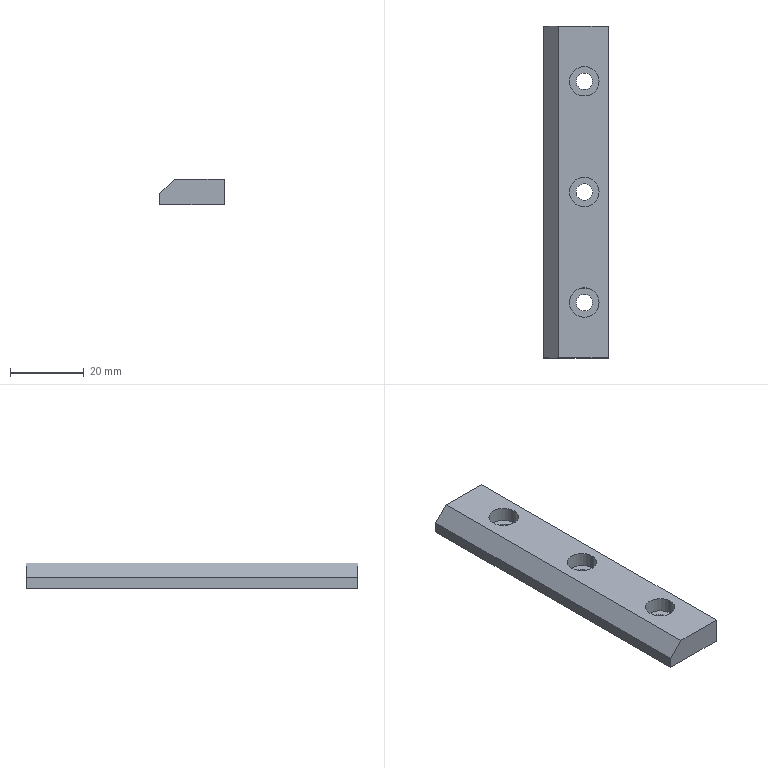Part | STEP file | detection slide seat cover plate--1 | 1 solid | 22 faces | box 17.5 x 90 x 7 mm | volume 9559 mm3 | cylinder 12 | plane 10 | commonest cylinder face diameters 4.5 x6 8 x6
STEP:
#1=CARTESIAN_POINT('',(0.,0.,0.));
#2=DIRECTION('',(0.,0.,1.));
#3=DIRECTION('',(1.,0.,0.));
#4=AXIS2_PLACEMENT_3D('',#1,#2,#3);
#5=CARTESIAN_POINT('',(7.648,22.1,3.));
#6=VERTEX_POINT('',#5);
#7=CARTESIAN_POINT('',(7.648,22.1,7.));
#8=VERTEX_POINT('',#7);
#9=CARTESIAN_POINT('',(7.648,22.1,3.));
#10=DIRECTION('',(0.,0.,1.));
#11=VECTOR('',#10,1.);
#12=LINE('',#9,#11);
#13=CARTESIAN_POINT('',(3.648,22.1,3.));
#14=DIRECTION('',(0.,0.,1.));
#15=DIRECTION('',(1.,0.,0.));
#16=AXIS2_PLACEMENT_3D('',#13,#14,#15);
#17=CYLINDRICAL_SURFACE('',#16,4.);
#18=CARTESIAN_POINT('',(6.283,0.));
#19=DIRECTION('',(0.,1.));
#20=VECTOR('',#19,1.);
#21=LINE('',#18,#20);
#22=(GEOMETRIC_REPRESENTATION_CONTEXT(2)PARAMETRIC_REPRESENTATION_CONTEXT()REPRESENTATION_CONTEXT('',''));
#23=DEFINITIONAL_REPRESENTATION('',(#21),#22);
#24=PCURVE('',#17,#23);
#25=CARTESIAN_POINT('',(3.648,22.1,3.));
#26=DIRECTION('',(0.,0.,1.));
#27=DIRECTION('',(1.,0.,0.));
#28=AXIS2_PLACEMENT_3D('',#25,#26,#27);
#29=CYLINDRICAL_SURFACE('',#28,4.);
#30=CARTESIAN_POINT('',(0.,0.));
#31=DIRECTION('',(0.,1.));
#32=VECTOR('',#31,1.);
#33=LINE('',#30,#32);
#34=(GEOMETRIC_REPRESENTATION_CONTEXT(2)PARAMETRIC_REPRESENTATION_CONTEXT()REPRESENTATION_CONTEXT('',''));
#35=DEFINITIONAL_REPRESENTATION('',(#33),#34);
#36=PCURVE('',#29,#35);
#37=SURFACE_CURVE('',#12,(#24,#36),.PCURVE_S1.);
#38=EDGE_CURVE('',#6,#8,#37,.T.);
#39=ORIENTED_EDGE('',*,*,#38,.T.);
#40=CARTESIAN_POINT('',(-0.3518,22.1,7.));
#41=VERTEX_POINT('',#40);
#42=CARTESIAN_POINT('',(3.648,22.1,7.));
#43=DIRECTION('',(0.,0.,1.));
#44=DIRECTION('',(1.,0.,0.));
#45=AXIS2_PLACEMENT_3D('',#42,#43,#44);
#46=CIRCLE('',#45,4.);
#47=CARTESIAN_POINT('',(0.,4.));
#48=DIRECTION('',(1.,0.));
#49=VECTOR('',#48,1.);
#50=LINE('',#47,#49);
#51=(GEOMETRIC_REPRESENTATION_CONTEXT(2)PARAMETRIC_REPRESENTATION_CONTEXT()REPRESENTATION_CONTEXT('',''));
#52=DEFINITIONAL_REPRESENTATION('',(#50),#51);
#53=PCURVE('',#17,#52);
#54=CARTESIAN_POINT('',(-7.352,-52.9,7.));
#55=DIRECTION('',(0.,0.,1.));
#56=DIRECTION('',(1.,0.,0.));
#57=AXIS2_PLACEMENT_3D('',#54,#55,#56);
#58=PLANE('',#57);
#59=CARTESIAN_POINT('',(11.,75.));
#60=DIRECTION('',(1.,0.));
#61=AXIS2_PLACEMENT_2D('',#59,#60);
#62=CIRCLE('',#61,4.);
#63=(GEOMETRIC_REPRESENTATION_CONTEXT(2)PARAMETRIC_REPRESENTATION_CONTEXT()REPRESENTATION_CONTEXT('',''));
#64=DEFINITIONAL_REPRESENTATION('',(#62),#63);
#65=PCURVE('',#58,#64);
#66=SURFACE_CURVE('',#46,(#53,#65),.PCURVE_S1.);
#67=EDGE_CURVE('',#41,#8,#66,.T.);
#68=ORIENTED_EDGE('',*,*,#67,.F.);
#69=CARTESIAN_POINT('',(-0.3518,22.1,3.));
#70=VERTEX_POINT('',#69);
#71=CARTESIAN_POINT('',(-0.3518,22.1,3.));
#72=DIRECTION('',(0.,0.,1.));
#73=VECTOR('',#72,1.);
#74=LINE('',#71,#73);
#75=CARTESIAN_POINT('',(3.142,0.));
#76=DIRECTION('',(0.,1.));
#77=VECTOR('',#76,1.);
#78=LINE('',#75,#77);
#79=(GEOMETRIC_REPRESENTATION_CONTEXT(2)PARAMETRIC_REPRESENTATION_CONTEXT()REPRESENTATION_CONTEXT('',''));
#80=DEFINITIONAL_REPRESENTATION('',(#78),#79);
#81=PCURVE('',#17,#80);
#82=CARTESIAN_POINT('',(3.142,0.));
#83=DIRECTION('',(0.,1.));
#84=VECTOR('',#83,1.);
#85=LINE('',#82,#84);
#86=(GEOMETRIC_REPRESENTATION_CONTEXT(2)PARAMETRIC_REPRESENTATION_CONTEXT()REPRESENTATION_CONTEXT('',''));
#87=DEFINITIONAL_REPRESENTATION('',(#85),#86);
#88=PCURVE('',#29,#87);
#89=SURFACE_CURVE('',#74,(#81,#88),.PCURVE_S1.);
#90=EDGE_CURVE('',#70,#41,#89,.T.);
#91=ORIENTED_EDGE('',*,*,#90,.F.);
#92=CARTESIAN_POINT('',(3.648,22.1,3.));
#93=DIRECTION('',(0.,0.,1.));
#94=DIRECTION('',(1.,0.,0.));
#95=AXIS2_PLACEMENT_3D('',#92,#93,#94);
#96=CIRCLE('',#95,4.);
#97=CARTESIAN_POINT('',(0.,0.));
#98=DIRECTION('',(1.,0.));
#99=VECTOR('',#98,1.);
#100=LINE('',#97,#99);
#101=(GEOMETRIC_REPRESENTATION_CONTEXT(2)PARAMETRIC_REPRESENTATION_CONTEXT()REPRESENTATION_CONTEXT('',''));
#102=DEFINITIONAL_REPRESENTATION('',(#100),#101);
#103=PCURVE('',#17,#102);
#104=CARTESIAN_POINT('',(3.648,22.1,3.));
#105=DIRECTION('',(0.,0.,1.));
#106=DIRECTION('',(1.,0.,0.));
#107=AXIS2_PLACEMENT_3D('',#104,#105,#106);
#108=PLANE('',#107);
#109=CARTESIAN_POINT('',(0.,0.));
#110=DIRECTION('',(1.,0.));
#111=AXIS2_PLACEMENT_2D('',#109,#110);
#112=CIRCLE('',#111,4.);
#113=(GEOMETRIC_REPRESENTATION_CONTEXT(2)PARAMETRIC_REPRESENTATION_CONTEXT()REPRESENTATION_CONTEXT('',''));
#114=DEFINITIONAL_REPRESENTATION('',(#112),#113);
#115=PCURVE('',#108,#114);
#116=SURFACE_CURVE('',#96,(#103,#115),.PCURVE_S1.);
#117=EDGE_CURVE('',#70,#6,#116,.T.);
#118=ORIENTED_EDGE('',*,*,#117,.T.);
#119=EDGE_LOOP('',(#39,#68,#91,#118));
#120=FACE_BOUND('',#119,.F.);
#121=ADVANCED_FACE('',(#120),#17,.F.);
#122=CARTESIAN_POINT('',(7.648,-7.9,3.));
#123=VERTEX_POINT('',#122);
#124=CARTESIAN_POINT('',(7.648,-7.9,7.));
#125=VERTEX_POINT('',#124);
#126=CARTESIAN_POINT('',(7.648,-7.9,3.));
#127=DIRECTION('',(0.,0.,1.));
#128=VECTOR('',#127,1.);
#129=LINE('',#126,#128);
#130=CARTESIAN_POINT('',(3.648,-7.9,3.));
#131=DIRECTION('',(0.,0.,1.));
#132=DIRECTION('',(1.,0.,0.));
#133=AXIS2_PLACEMENT_3D('',#130,#131,#132);
#134=CYLINDRICAL_SURFACE('',#133,4.);
#135=CARTESIAN_POINT('',(6.283,0.));
#136=DIRECTION('',(0.,1.));
#137=VECTOR('',#136,1.);
#138=LINE('',#135,#137);
#139=(GEOMETRIC_REPRESENTATION_CONTEXT(2)PARAMETRIC_REPRESENTATION_CONTEXT()REPRESENTATION_CONTEXT('',''));
#140=DEFINITIONAL_REPRESENTATION('',(#138),#139);
#141=PCURVE('',#134,#140);
#142=CARTESIAN_POINT('',(3.648,-7.9,3.));
#143=DIRECTION('',(0.,0.,1.));
#144=DIRECTION('',(1.,0.,0.));
#145=AXIS2_PLACEMENT_3D('',#142,#143,#144);
#146=CYLINDRICAL_SURFACE('',#145,4.);
#147=CARTESIAN_POINT('',(0.,0.));
#148=DIRECTION('',(0.,1.));
#149=VECTOR('',#148,1.);
#150=LINE('',#147,#149);
#151=(GEOMETRIC_REPRESENTATION_CONTEXT(2)PARAMETRIC_REPRESENTATION_CONTEXT()REPRESENTATION_CONTEXT('',''));
#152=DEFINITIONAL_REPRESENTATION('',(#150),#151);
#153=PCURVE('',#146,#152);
#154=SURFACE_CURVE('',#129,(#141,#153),.PCURVE_S1.);
#155=EDGE_CURVE('',#123,#125,#154,.T.);
#156=ORIENTED_EDGE('',*,*,#155,.T.);
#157=CARTESIAN_POINT('',(-0.3518,-7.9,7.));
#158=VERTEX_POINT('',#157);
#159=CARTESIAN_POINT('',(3.648,-7.9,7.));
#160=DIRECTION('',(0.,0.,1.));
#161=DIRECTION('',(1.,0.,0.));
#162=AXIS2_PLACEMENT_3D('',#159,#160,#161);
#163=CIRCLE('',#162,4.);
#164=CARTESIAN_POINT('',(0.,4.));
#165=DIRECTION('',(1.,0.));
#166=VECTOR('',#165,1.);
#167=LINE('',#164,#166);
#168=(GEOMETRIC_REPRESENTATION_CONTEXT(2)PARAMETRIC_REPRESENTATION_CONTEXT()REPRESENTATION_CONTEXT('',''));
#169=DEFINITIONAL_REPRESENTATION('',(#167),#168);
#170=PCURVE('',#134,#169);
#171=CARTESIAN_POINT('',(11.,45.));
#172=DIRECTION('',(1.,0.));
#173=AXIS2_PLACEMENT_2D('',#171,#172);
#174=CIRCLE('',#173,4.);
#175=(GEOMETRIC_REPRESENTATION_CONTEXT(2)PARAMETRIC_REPRESENTATION_CONTEXT()REPRESENTATION_CONTEXT('',''));
#176=DEFINITIONAL_REPRESENTATION('',(#174),#175);
#177=PCURVE('',#58,#176);
#178=SURFACE_CURVE('',#163,(#170,#177),.PCURVE_S1.);
#179=EDGE_CURVE('',#158,#125,#178,.T.);
#180=ORIENTED_EDGE('',*,*,#179,.F.);
#181=CARTESIAN_POINT('',(-0.3518,-7.9,3.));
#182=VERTEX_POINT('',#181);
#183=CARTESIAN_POINT('',(-0.3518,-7.9,3.));
#184=DIRECTION('',(0.,0.,1.));
#185=VECTOR('',#184,1.);
#186=LINE('',#183,#185);
#187=CARTESIAN_POINT('',(3.142,0.));
#188=DIRECTION('',(0.,1.));
#189=VECTOR('',#188,1.);
#190=LINE('',#187,#189);
#191=(GEOMETRIC_REPRESENTATION_CONTEXT(2)PARAMETRIC_REPRESENTATION_CONTEXT()REPRESENTATION_CONTEXT('',''));
#192=DEFINITIONAL_REPRESENTATION('',(#190),#191);
#193=PCURVE('',#134,#192);
#194=CARTESIAN_POINT('',(3.142,0.));
#195=DIRECTION('',(0.,1.));
#196=VECTOR('',#195,1.);
#197=LINE('',#194,#196);
#198=(GEOMETRIC_REPRESENTATION_CONTEXT(2)PARAMETRIC_REPRESENTATION_CONTEXT()REPRESENTATION_CONTEXT('',''));
#199=DEFINITIONAL_REPRESENTATION('',(#197),#198);
#200=PCURVE('',#146,#199);
#201=SURFACE_CURVE('',#186,(#193,#200),.PCURVE_S1.);
#202=EDGE_CURVE('',#182,#158,#201,.T.);
#203=ORIENTED_EDGE('',*,*,#202,.F.);
#204=CARTESIAN_POINT('',(3.648,-7.9,3.));
#205=DIRECTION('',(0.,0.,1.));
#206=DIRECTION('',(1.,0.,0.));
#207=AXIS2_PLACEMENT_3D('',#204,#205,#206);
#208=CIRCLE('',#207,4.);
#209=CARTESIAN_POINT('',(0.,0.));
#210=DIRECTION('',(1.,0.));
#211=VECTOR('',#210,1.);
#212=LINE('',#209,#211);
#213=(GEOMETRIC_REPRESENTATION_CONTEXT(2)PARAMETRIC_REPRESENTATION_CONTEXT()REPRESENTATION_CONTEXT('',''));
#214=DEFINITIONAL_REPRESENTATION('',(#212),#213);
#215=PCURVE('',#134,#214);
#216=CARTESIAN_POINT('',(3.648,-7.9,3.));
#217=DIRECTION('',(0.,0.,1.));
#218=DIRECTION('',(1.,0.,0.));
#219=AXIS2_PLACEMENT_3D('',#216,#217,#218);
#220=PLANE('',#219);
#221=CARTESIAN_POINT('',(0.,0.));
#222=DIRECTION('',(1.,0.));
#223=AXIS2_PLACEMENT_2D('',#221,#222);
#224=CIRCLE('',#223,4.);
#225=(GEOMETRIC_REPRESENTATION_CONTEXT(2)PARAMETRIC_REPRESENTATION_CONTEXT()REPRESENTATION_CONTEXT('',''));
#226=DEFINITIONAL_REPRESENTATION('',(#224),#225);
#227=PCURVE('',#220,#226);
#228=SURFACE_CURVE('',#208,(#215,#227),.PCURVE_S1.);
#229=EDGE_CURVE('',#182,#123,#228,.T.);
#230=ORIENTED_EDGE('',*,*,#229,.T.);
#231=EDGE_LOOP('',(#156,#180,#203,#230));
#232=FACE_BOUND('',#231,.F.);
#233=ADVANCED_FACE('',(#232),#134,.F.);
#234=CARTESIAN_POINT('',(7.648,-37.9,3.));
#235=VERTEX_POINT('',#234);
#236=CARTESIAN_POINT('',(7.648,-37.9,7.));
#237=VERTEX_POINT('',#236);
#238=CARTESIAN_POINT('',(7.648,-37.9,3.));
#239=DIRECTION('',(0.,0.,1.));
#240=VECTOR('',#239,1.);
#241=LINE('',#238,#240);
#242=CARTESIAN_POINT('',(3.648,-37.9,3.));
#243=DIRECTION('',(0.,0.,1.));
#244=DIRECTION('',(1.,0.,0.));
#245=AXIS2_PLACEMENT_3D('',#242,#243,#244);
#246=CYLINDRICAL_SURFACE('',#245,4.);
#247=CARTESIAN_POINT('',(6.283,0.));
#248=DIRECTION('',(0.,1.));
#249=VECTOR('',#248,1.);
#250=LINE('',#247,#249);
#251=(GEOMETRIC_REPRESENTATION_CONTEXT(2)PARAMETRIC_REPRESENTATION_CONTEXT()REPRESENTATION_CONTEXT('',''));
#252=DEFINITIONAL_REPRESENTATION('',(#250),#251);
#253=PCURVE('',#246,#252);
#254=CARTESIAN_POINT('',(3.648,-37.9,3.));
#255=DIRECTION('',(0.,0.,1.));
#256=DIRECTION('',(1.,0.,0.));
#257=AXIS2_PLACEMENT_3D('',#254,#255,#256);
#258=CYLINDRICAL_SURFACE('',#257,4.);
#259=CARTESIAN_POINT('',(0.,0.));
#260=DIRECTION('',(0.,1.));
#261=VECTOR('',#260,1.);
#262=LINE('',#259,#261);
#263=(GEOMETRIC_REPRESENTATION_CONTEXT(2)PARAMETRIC_REPRESENTATION_CONTEXT()REPRESENTATION_CONTEXT('',''));
#264=DEFINITIONAL_REPRESENTATION('',(#262),#263);
#265=PCURVE('',#258,#264);
#266=SURFACE_CURVE('',#241,(#253,#265),.PCURVE_S1.);
#267=EDGE_CURVE('',#235,#237,#266,.T.);
#268=ORIENTED_EDGE('',*,*,#267,.T.);
#269=CARTESIAN_POINT('',(-0.3518,-37.9,7.));
#270=VERTEX_POINT('',#269);
#271=CARTESIAN_POINT('',(3.648,-37.9,7.));
#272=DIRECTION('',(0.,0.,1.));
#273=DIRECTION('',(1.,0.,0.));
#274=AXIS2_PLACEMENT_3D('',#271,#272,#273);
#275=CIRCLE('',#274,4.);
#276=CARTESIAN_POINT('',(0.,4.));
#277=DIRECTION('',(1.,0.));
#278=VECTOR('',#277,1.);
#279=LINE('',#276,#278);
#280=(GEOMETRIC_REPRESENTATION_CONTEXT(2)PARAMETRIC_REPRESENTATION_CONTEXT()REPRESENTATION_CONTEXT('',''));
#281=DEFINITIONAL_REPRESENTATION('',(#279),#280);
#282=PCURVE('',#246,#281);
#283=CARTESIAN_POINT('',(11.,15.));
#284=DIRECTION('',(1.,0.));
#285=AXIS2_PLACEMENT_2D('',#283,#284);
#286=CIRCLE('',#285,4.);
#287=(GEOMETRIC_REPRESENTATION_CONTEXT(2)PARAMETRIC_REPRESENTATION_CONTEXT()REPRESENTATION_CONTEXT('',''));
#288=DEFINITIONAL_REPRESENTATION('',(#286),#287);
#289=PCURVE('',#58,#288);
#290=SURFACE_CURVE('',#275,(#282,#289),.PCURVE_S1.);
#291=EDGE_CURVE('',#270,#237,#290,.T.);
#292=ORIENTED_EDGE('',*,*,#291,.F.);
#293=CARTESIAN_POINT('',(-0.3518,-37.9,3.));
#294=VERTEX_POINT('',#293);
#295=CARTESIAN_POINT('',(-0.3518,-37.9,3.));
#296=DIRECTION('',(0.,0.,1.));
#297=VECTOR('',#296,1.);
#298=LINE('',#295,#297);
#299=CARTESIAN_POINT('',(3.142,0.));
#300=DIRECTION('',(0.,1.));
#301=VECTOR('',#300,1.);
#302=LINE('',#299,#301);
#303=(GEOMETRIC_REPRESENTATION_CONTEXT(2)PARAMETRIC_REPRESENTATION_CONTEXT()REPRESENTATION_CONTEXT('',''));
#304=DEFINITIONAL_REPRESENTATION('',(#302),#303);
#305=PCURVE('',#246,#304);
#306=CARTESIAN_POINT('',(3.142,0.));
#307=DIRECTION('',(0.,1.));
#308=VECTOR('',#307,1.);
#309=LINE('',#306,#308);
#310=(GEOMETRIC_REPRESENTATION_CONTEXT(2)PARAMETRIC_REPRESENTATION_CONTEXT()REPRESENTATION_CONTEXT('',''));
#311=DEFINITIONAL_REPRESENTATION('',(#309),#310);
#312=PCURVE('',#258,#311);
#313=SURFACE_CURVE('',#298,(#305,#312),.PCURVE_S1.);
#314=EDGE_CURVE('',#294,#270,#313,.T.);
#315=ORIENTED_EDGE('',*,*,#314,.F.);
#316=CARTESIAN_POINT('',(3.648,-37.9,3.));
#317=DIRECTION('',(0.,0.,1.));
#318=DIRECTION('',(1.,0.,0.));
#319=AXIS2_PLACEMENT_3D('',#316,#317,#318);
#320=CIRCLE('',#319,4.);
#321=CARTESIAN_POINT('',(0.,0.));
#322=DIRECTION('',(1.,0.));
#323=VECTOR('',#322,1.);
#324=LINE('',#321,#323);
#325=(GEOMETRIC_REPRESENTATION_CONTEXT(2)PARAMETRIC_REPRESENTATION_CONTEXT()REPRESENTATION_CONTEXT('',''));
#326=DEFINITIONAL_REPRESENTATION('',(#324),#325);
#327=PCURVE('',#246,#326);
#328=CARTESIAN_POINT('',(3.648,-37.9,3.));
#329=DIRECTION('',(0.,0.,1.));
#330=DIRECTION('',(1.,0.,0.));
#331=AXIS2_PLACEMENT_3D('',#328,#329,#330);
#332=PLANE('',#331);
#333=CARTESIAN_POINT('',(0.,0.));
#334=DIRECTION('',(1.,0.));
#335=AXIS2_PLACEMENT_2D('',#333,#334);
#336=CIRCLE('',#335,4.);
#337=(GEOMETRIC_REPRESENTATION_CONTEXT(2)PARAMETRIC_REPRESENTATION_CONTEXT()REPRESENTATION_CONTEXT('',''));
#338=DEFINITIONAL_REPRESENTATION('',(#336),#337);
#339=PCURVE('',#332,#338);
#340=SURFACE_CURVE('',#320,(#327,#339),.PCURVE_S1.);
#341=EDGE_CURVE('',#294,#235,#340,.T.);
#342=ORIENTED_EDGE('',*,*,#341,.T.);
#343=EDGE_LOOP('',(#268,#292,#315,#342));
#344=FACE_BOUND('',#343,.F.);
#345=ADVANCED_FACE('',(#344),#246,.F.);
#346=CARTESIAN_POINT('',(1.398,-37.9,3.));
#347=VERTEX_POINT('',#346);
#348=CARTESIAN_POINT('',(1.398,-37.9,0.));
#349=VERTEX_POINT('',#348);
#350=CARTESIAN_POINT('',(1.398,-37.9,7.));
#351=DIRECTION('',(0.,0.,-1.));
#352=VECTOR('',#351,1.);
#353=LINE('',#350,#352);
#354=CARTESIAN_POINT('',(3.648,-37.9,7.));
#355=DIRECTION('',(0.,0.,-1.));
#356=DIRECTION('',(-1.,0.,0.));
#357=AXIS2_PLACEMENT_3D('',#354,#355,#356);
#358=CYLINDRICAL_SURFACE('',#357,2.25);
#359=CARTESIAN_POINT('',(6.283,0.));
#360=DIRECTION('',(0.,1.));
#361=VECTOR('',#360,1.);
#362=LINE('',#359,#361);
#363=(GEOMETRIC_REPRESENTATION_CONTEXT(2)PARAMETRIC_REPRESENTATION_CONTEXT()REPRESENTATION_CONTEXT('',''));
#364=DEFINITIONAL_REPRESENTATION('',(#362),#363);
#365=PCURVE('',#358,#364);
#366=CARTESIAN_POINT('',(3.648,-37.9,7.));
#367=DIRECTION('',(0.,0.,-1.));
#368=DIRECTION('',(-1.,0.,0.));
#369=AXIS2_PLACEMENT_3D('',#366,#367,#368);
#370=CYLINDRICAL_SURFACE('',#369,2.25);
#371=CARTESIAN_POINT('',(0.,0.));
#372=DIRECTION('',(0.,1.));
#373=VECTOR('',#372,1.);
#374=LINE('',#371,#373);
#375=(GEOMETRIC_REPRESENTATION_CONTEXT(2)PARAMETRIC_REPRESENTATION_CONTEXT()REPRESENTATION_CONTEXT('',''));
#376=DEFINITIONAL_REPRESENTATION('',(#374),#375);
#377=PCURVE('',#370,#376);
#378=SURFACE_CURVE('',#353,(#365,#377),.PCURVE_S1.);
#379=EDGE_CURVE('',#347,#349,#378,.T.);
#380=ORIENTED_EDGE('',*,*,#379,.T.);
#381=CARTESIAN_POINT('',(5.898,-37.9,0.));
#382=VERTEX_POINT('',#381);
#383=CARTESIAN_POINT('',(3.648,-37.9,0.));
#384=DIRECTION('',(0.,0.,1.));
#385=DIRECTION('',(1.,0.,0.));
#386=AXIS2_PLACEMENT_3D('',#383,#384,#385);
#387=CIRCLE('',#386,2.25);
#388=CARTESIAN_POINT('',(9.425,7.));
#389=DIRECTION('',(-1.,0.));
#390=VECTOR('',#389,1.);
#391=LINE('',#388,#390);
#392=(GEOMETRIC_REPRESENTATION_CONTEXT(2)PARAMETRIC_REPRESENTATION_CONTEXT()REPRESENTATION_CONTEXT('',''));
#393=DEFINITIONAL_REPRESENTATION('',(#391),#392);
#394=PCURVE('',#358,#393);
#395=CARTESIAN_POINT('',(-7.352,-52.9,0.));
#396=DIRECTION('',(0.,0.,1.));
#397=DIRECTION('',(1.,0.,0.));
#398=AXIS2_PLACEMENT_3D('',#395,#396,#397);
#399=PLANE('',#398);
#400=CARTESIAN_POINT('',(11.,15.));
#401=DIRECTION('',(1.,0.));
#402=AXIS2_PLACEMENT_2D('',#400,#401);
#403=CIRCLE('',#402,2.25);
#404=(GEOMETRIC_REPRESENTATION_CONTEXT(2)PARAMETRIC_REPRESENTATION_CONTEXT()REPRESENTATION_CONTEXT('',''));
#405=DEFINITIONAL_REPRESENTATION('',(#403),#404);
#406=PCURVE('',#399,#405);
#407=SURFACE_CURVE('',#387,(#394,#406),.PCURVE_S1.);
#408=EDGE_CURVE('',#349,#382,#407,.T.);
#409=ORIENTED_EDGE('',*,*,#408,.T.);
#410=CARTESIAN_POINT('',(5.898,-37.9,3.));
#411=VERTEX_POINT('',#410);
#412=CARTESIAN_POINT('',(5.898,-37.9,7.));
#413=DIRECTION('',(0.,0.,-1.));
#414=VECTOR('',#413,1.);
#415=LINE('',#412,#414);
#416=CARTESIAN_POINT('',(3.142,0.));
#417=DIRECTION('',(0.,1.));
#418=VECTOR('',#417,1.);
#419=LINE('',#416,#418);
#420=(GEOMETRIC_REPRESENTATION_CONTEXT(2)PARAMETRIC_REPRESENTATION_CONTEXT()REPRESENTATION_CONTEXT('',''));
#421=DEFINITIONAL_REPRESENTATION('',(#419),#420);
#422=PCURVE('',#358,#421);
#423=CARTESIAN_POINT('',(3.142,0.));
#424=DIRECTION('',(0.,1.));
#425=VECTOR('',#424,1.);
#426=LINE('',#423,#425);
#427=(GEOMETRIC_REPRESENTATION_CONTEXT(2)PARAMETRIC_REPRESENTATION_CONTEXT()REPRESENTATION_CONTEXT('',''));
#428=DEFINITIONAL_REPRESENTATION('',(#426),#427);
#429=PCURVE('',#370,#428);
#430=SURFACE_CURVE('',#415,(#422,#429),.PCURVE_S1.);
#431=EDGE_CURVE('',#411,#382,#430,.T.);
#432=ORIENTED_EDGE('',*,*,#431,.F.);
#433=CARTESIAN_POINT('',(3.648,-37.9,3.));
#434=DIRECTION('',(0.,0.,1.));
#435=DIRECTION('',(1.,0.,0.));
#436=AXIS2_PLACEMENT_3D('',#433,#434,#435);
#437=CIRCLE('',#436,2.25);
#438=CARTESIAN_POINT('',(9.425,4.));
#439=DIRECTION('',(-1.,0.));
#440=VECTOR('',#439,1.);
#441=LINE('',#438,#440);
#442=(GEOMETRIC_REPRESENTATION_CONTEXT(2)PARAMETRIC_REPRESENTATION_CONTEXT()REPRESENTATION_CONTEXT('',''));
#443=DEFINITIONAL_REPRESENTATION('',(#441),#442);
#444=PCURVE('',#358,#443);
#445=CARTESIAN_POINT('',(0.,0.));
#446=DIRECTION('',(1.,0.));
#447=AXIS2_PLACEMENT_2D('',#445,#446);
#448=CIRCLE('',#447,2.25);
#449=(GEOMETRIC_REPRESENTATION_CONTEXT(2)PARAMETRIC_REPRESENTATION_CONTEXT()REPRESENTATION_CONTEXT('',''));
#450=DEFINITIONAL_REPRESENTATION('',(#448),#449);
#451=PCURVE('',#332,#450);
#452=SURFACE_CURVE('',#437,(#444,#451),.PCURVE_S1.);
#453=EDGE_CURVE('',#347,#411,#452,.T.);
#454=ORIENTED_EDGE('',*,*,#453,.F.);
#455=EDGE_LOOP('',(#380,#409,#432,#454));
#456=FACE_BOUND('',#455,.F.);
#457=ADVANCED_FACE('',(#456),#358,.F.);
#458=CARTESIAN_POINT('',(1.398,-7.9,3.));
#459=VERTEX_POINT('',#458);
#460=CARTESIAN_POINT('',(1.398,-7.9,0.));
#461=VERTEX_POINT('',#460);
#462=CARTESIAN_POINT('',(1.398,-7.9,7.));
#463=DIRECTION('',(0.,0.,-1.));
#464=VECTOR('',#463,1.);
#465=LINE('',#462,#464);
#466=CARTESIAN_POINT('',(3.648,-7.9,7.));
#467=DIRECTION('',(0.,0.,-1.));
#468=DIRECTION('',(-1.,0.,0.));
#469=AXIS2_PLACEMENT_3D('',#466,#467,#468);
#470=CYLINDRICAL_SURFACE('',#469,2.25);
#471=CARTESIAN_POINT('',(6.283,0.));
#472=DIRECTION('',(0.,1.));
#473=VECTOR('',#472,1.);
#474=LINE('',#471,#473);
#475=(GEOMETRIC_REPRESENTATION_CONTEXT(2)PARAMETRIC_REPRESENTATION_CONTEXT()REPRESENTATION_CONTEXT('',''));
#476=DEFINITIONAL_REPRESENTATION('',(#474),#475);
#477=PCURVE('',#470,#476);
#478=CARTESIAN_POINT('',(3.648,-7.9,7.));
#479=DIRECTION('',(0.,0.,-1.));
#480=DIRECTION('',(-1.,0.,0.));
#481=AXIS2_PLACEMENT_3D('',#478,#479,#480);
#482=CYLINDRICAL_SURFACE('',#481,2.25);
#483=CARTESIAN_POINT('',(0.,0.));
#484=DIRECTION('',(0.,1.));
#485=VECTOR('',#484,1.);
#486=LINE('',#483,#485);
#487=(GEOMETRIC_REPRESENTATION_CONTEXT(2)PARAMETRIC_REPRESENTATION_CONTEXT()REPRESENTATION_CONTEXT('',''));
#488=DEFINITIONAL_REPRESENTATION('',(#486),#487);
#489=PCURVE('',#482,#488);
#490=SURFACE_CURVE('',#465,(#477,#489),.PCURVE_S1.);
#491=EDGE_CURVE('',#459,#461,#490,.T.);
#492=ORIENTED_EDGE('',*,*,#491,.T.);
#493=CARTESIAN_POINT('',(5.898,-7.9,0.));
#494=VERTEX_POINT('',#493);
#495=CARTESIAN_POINT('',(3.648,-7.9,0.));
#496=DIRECTION('',(0.,0.,1.));
#497=DIRECTION('',(1.,0.,0.));
#498=AXIS2_PLACEMENT_3D('',#495,#496,#497);
#499=CIRCLE('',#498,2.25);
#500=CARTESIAN_POINT('',(9.425,7.));
#501=DIRECTION('',(-1.,0.));
#502=VECTOR('',#501,1.);
#503=LINE('',#500,#502);
#504=(GEOMETRIC_REPRESENTATION_CONTEXT(2)PARAMETRIC_REPRESENTATION_CONTEXT()REPRESENTATION_CONTEXT('',''));
#505=DEFINITIONAL_REPRESENTATION('',(#503),#504);
#506=PCURVE('',#470,#505);
#507=CARTESIAN_POINT('',(11.,45.));
#508=DIRECTION('',(1.,0.));
#509=AXIS2_PLACEMENT_2D('',#507,#508);
#510=CIRCLE('',#509,2.25);
#511=(GEOMETRIC_REPRESENTATION_CONTEXT(2)PARAMETRIC_REPRESENTATION_CONTEXT()REPRESENTATION_CONTEXT('',''));
#512=DEFINITIONAL_REPRESENTATION('',(#510),#511);
#513=PCURVE('',#399,#512);
#514=SURFACE_CURVE('',#499,(#506,#513),.PCURVE_S1.);
#515=EDGE_CURVE('',#461,#494,#514,.T.);
#516=ORIENTED_EDGE('',*,*,#515,.T.);
#517=CARTESIAN_POINT('',(5.898,-7.9,3.));
#518=VERTEX_POINT('',#517);
#519=CARTESIAN_POINT('',(5.898,-7.9,7.));
#520=DIRECTION('',(0.,0.,-1.));
#521=VECTOR('',#520,1.);
#522=LINE('',#519,#521);
#523=CARTESIAN_POINT('',(3.142,0.));
#524=DIRECTION('',(0.,1.));
#525=VECTOR('',#524,1.);
#526=LINE('',#523,#525);
#527=(GEOMETRIC_REPRESENTATION_CONTEXT(2)PARAMETRIC_REPRESENTATION_CONTEXT()REPRESENTATION_CONTEXT('',''));
#528=DEFINITIONAL_REPRESENTATION('',(#526),#527);
#529=PCURVE('',#470,#528);
#530=CARTESIAN_POINT('',(3.142,0.));
#531=DIRECTION('',(0.,1.));
#532=VECTOR('',#531,1.);
#533=LINE('',#530,#532);
#534=(GEOMETRIC_REPRESENTATION_CONTEXT(2)PARAMETRIC_REPRESENTATION_CONTEXT()REPRESENTATION_CONTEXT('',''));
#535=DEFINITIONAL_REPRESENTATION('',(#533),#534);
#536=PCURVE('',#482,#535);
#537=SURFACE_CURVE('',#522,(#529,#536),.PCURVE_S1.);
#538=EDGE_CURVE('',#518,#494,#537,.T.);
#539=ORIENTED_EDGE('',*,*,#538,.F.);
#540=CARTESIAN_POINT('',(3.648,-7.9,3.));
#541=DIRECTION('',(0.,0.,1.));
#542=DIRECTION('',(1.,0.,0.));
#543=AXIS2_PLACEMENT_3D('',#540,#541,#542);
#544=CIRCLE('',#543,2.25);
#545=CARTESIAN_POINT('',(9.425,4.));
#546=DIRECTION('',(-1.,0.));
#547=VECTOR('',#546,1.);
#548=LINE('',#545,#547);
#549=(GEOMETRIC_REPRESENTATION_CONTEXT(2)PARAMETRIC_REPRESENTATION_CONTEXT()REPRESENTATION_CONTEXT('',''));
#550=DEFINITIONAL_REPRESENTATION('',(#548),#549);
#551=PCURVE('',#470,#550);
#552=CARTESIAN_POINT('',(0.,0.));
#553=DIRECTION('',(1.,0.));
#554=AXIS2_PLACEMENT_2D('',#552,#553);
#555=CIRCLE('',#554,2.25);
#556=(GEOMETRIC_REPRESENTATION_CONTEXT(2)PARAMETRIC_REPRESENTATION_CONTEXT()REPRESENTATION_CONTEXT('',''));
#557=DEFINITIONAL_REPRESENTATION('',(#555),#556);
#558=PCURVE('',#220,#557);
#559=SURFACE_CURVE('',#544,(#551,#558),.PCURVE_S1.);
#560=EDGE_CURVE('',#459,#518,#559,.T.);
#561=ORIENTED_EDGE('',*,*,#560,.F.);
#562=EDGE_LOOP('',(#492,#516,#539,#561));
#563=FACE_BOUND('',#562,.F.);
#564=ADVANCED_FACE('',(#563),#470,.F.);
#565=CARTESIAN_POINT('',(1.398,22.1,3.));
#566=VERTEX_POINT('',#565);
#567=CARTESIAN_POINT('',(1.398,22.1,0.));
#568=VERTEX_POINT('',#567);
#569=CARTESIAN_POINT('',(1.398,22.1,7.));
#570=DIRECTION('',(0.,0.,-1.));
#571=VECTOR('',#570,1.);
#572=LINE('',#569,#571);
#573=CARTESIAN_POINT('',(3.648,22.1,7.));
#574=DIRECTION('',(0.,0.,-1.));
#575=DIRECTION('',(-1.,0.,0.));
#576=AXIS2_PLACEMENT_3D('',#573,#574,#575);
#577=CYLINDRICAL_SURFACE('',#576,2.25);
#578=CARTESIAN_POINT('',(6.283,0.));
#579=DIRECTION('',(0.,1.));
#580=VECTOR('',#579,1.);
#581=LINE('',#578,#580);
#582=(GEOMETRIC_REPRESENTATION_CONTEXT(2)PARAMETRIC_REPRESENTATION_CONTEXT()REPRESENTATION_CONTEXT('',''));
#583=DEFINITIONAL_REPRESENTATION('',(#581),#582);
#584=PCURVE('',#577,#583);
#585=CARTESIAN_POINT('',(3.648,22.1,7.));
#586=DIRECTION('',(0.,0.,-1.));
#587=DIRECTION('',(-1.,0.,0.));
#588=AXIS2_PLACEMENT_3D('',#585,#586,#587);
#589=CYLINDRICAL_SURFACE('',#588,2.25);
#590=CARTESIAN_POINT('',(0.,0.));
#591=DIRECTION('',(0.,1.));
#592=VECTOR('',#591,1.);
#593=LINE('',#590,#592);
#594=(GEOMETRIC_REPRESENTATION_CONTEXT(2)PARAMETRIC_REPRESENTATION_CONTEXT()REPRESENTATION_CONTEXT('',''));
#595=DEFINITIONAL_REPRESENTATION('',(#593),#594);
#596=PCURVE('',#589,#595);
#597=SURFACE_CURVE('',#572,(#584,#596),.PCURVE_S1.);
#598=EDGE_CURVE('',#566,#568,#597,.T.);
#599=ORIENTED_EDGE('',*,*,#598,.T.);
#600=CARTESIAN_POINT('',(5.898,22.1,0.));
#601=VERTEX_POINT('',#600);
#602=CARTESIAN_POINT('',(3.648,22.1,0.));
#603=DIRECTION('',(0.,0.,1.));
#604=DIRECTION('',(1.,0.,0.));
#605=AXIS2_PLACEMENT_3D('',#602,#603,#604);
#606=CIRCLE('',#605,2.25);
#607=CARTESIAN_POINT('',(9.425,7.));
#608=DIRECTION('',(-1.,0.));
#609=VECTOR('',#608,1.);
#610=LINE('',#607,#609);
#611=(GEOMETRIC_REPRESENTATION_CONTEXT(2)PARAMETRIC_REPRESENTATION_CONTEXT()REPRESENTATION_CONTEXT('',''));
#612=DEFINITIONAL_REPRESENTATION('',(#610),#611);
#613=PCURVE('',#577,#612);
#614=CARTESIAN_POINT('',(11.,75.));
#615=DIRECTION('',(1.,0.));
#616=AXIS2_PLACEMENT_2D('',#614,#615);
#617=CIRCLE('',#616,2.25);
#618=(GEOMETRIC_REPRESENTATION_CONTEXT(2)PARAMETRIC_REPRESENTATION_CONTEXT()REPRESENTATION_CONTEXT('',''));
#619=DEFINITIONAL_REPRESENTATION('',(#617),#618);
#620=PCURVE('',#399,#619);
#621=SURFACE_CURVE('',#606,(#613,#620),.PCURVE_S1.);
#622=EDGE_CURVE('',#568,#601,#621,.T.);
#623=ORIENTED_EDGE('',*,*,#622,.T.);
#624=CARTESIAN_POINT('',(5.898,22.1,3.));
#625=VERTEX_POINT('',#624);
#626=CARTESIAN_POINT('',(5.898,22.1,7.));
#627=DIRECTION('',(0.,0.,-1.));
#628=VECTOR('',#627,1.);
#629=LINE('',#626,#628);
#630=CARTESIAN_POINT('',(3.142,0.));
#631=DIRECTION('',(0.,1.));
#632=VECTOR('',#631,1.);
#633=LINE('',#630,#632);
#634=(GEOMETRIC_REPRESENTATION_CONTEXT(2)PARAMETRIC_REPRESENTATION_CONTEXT()REPRESENTATION_CONTEXT('',''));
#635=DEFINITIONAL_REPRESENTATION('',(#633),#634);
#636=PCURVE('',#577,#635);
#637=CARTESIAN_POINT('',(3.142,0.));
#638=DIRECTION('',(0.,1.));
#639=VECTOR('',#638,1.);
#640=LINE('',#637,#639);
#641=(GEOMETRIC_REPRESENTATION_CONTEXT(2)PARAMETRIC_REPRESENTATION_CONTEXT()REPRESENTATION_CONTEXT('',''));
#642=DEFINITIONAL_REPRESENTATION('',(#640),#641);
#643=PCURVE('',#589,#642);
#644=SURFACE_CURVE('',#629,(#636,#643),.PCURVE_S1.);
#645=EDGE_CURVE('',#625,#601,#644,.T.);
#646=ORIENTED_EDGE('',*,*,#645,.F.);
#647=CARTESIAN_POINT('',(3.648,22.1,3.));
#648=DIRECTION('',(0.,0.,1.));
#649=DIRECTION('',(1.,0.,0.));
#650=AXIS2_PLACEMENT_3D('',#647,#648,#649);
#651=CIRCLE('',#650,2.25);
#652=CARTESIAN_POINT('',(9.425,4.));
#653=DIRECTION('',(-1.,0.));
#654=VECTOR('',#653,1.);
#655=LINE('',#652,#654);
#656=(GEOMETRIC_REPRESENTATION_CONTEXT(2)PARAMETRIC_REPRESENTATION_CONTEXT()REPRESENTATION_CONTEXT('',''));
#657=DEFINITIONAL_REPRESENTATION('',(#655),#656);
#658=PCURVE('',#577,#657);
#659=CARTESIAN_POINT('',(0.,0.));
#660=DIRECTION('',(1.,0.));
#661=AXIS2_PLACEMENT_2D('',#659,#660);
#662=CIRCLE('',#661,2.25);
#663=(GEOMETRIC_REPRESENTATION_CONTEXT(2)PARAMETRIC_REPRESENTATION_CONTEXT()REPRESENTATION_CONTEXT('',''));
#664=DEFINITIONAL_REPRESENTATION('',(#662),#663);
#665=PCURVE('',#108,#664);
#666=SURFACE_CURVE('',#651,(#658,#665),.PCURVE_S1.);
#667=EDGE_CURVE('',#566,#625,#666,.T.);
#668=ORIENTED_EDGE('',*,*,#667,.F.);
#669=EDGE_LOOP('',(#599,#623,#646,#668));
#670=FACE_BOUND('',#669,.F.);
#671=ADVANCED_FACE('',(#670),#577,.F.);
#672=CARTESIAN_POINT('',(3.648,22.1,0.));
#673=DIRECTION('',(0.,0.,1.));
#674=DIRECTION('',(1.,0.,0.));
#675=AXIS2_PLACEMENT_3D('',#672,#673,#674);
#676=CIRCLE('',#675,2.25);
#677=CARTESIAN_POINT('',(3.142,7.));
#678=DIRECTION('',(-1.,0.));
#679=VECTOR('',#678,1.);
#680=LINE('',#677,#679);
#681=(GEOMETRIC_REPRESENTATION_CONTEXT(2)PARAMETRIC_REPRESENTATION_CONTEXT()REPRESENTATION_CONTEXT('',''));
#682=DEFINITIONAL_REPRESENTATION('',(#680),#681);
#683=PCURVE('',#589,#682);
#684=CARTESIAN_POINT('',(11.,75.));
#685=DIRECTION('',(1.,0.));
#686=AXIS2_PLACEMENT_2D('',#684,#685);
#687=CIRCLE('',#686,2.25);
#688=(GEOMETRIC_REPRESENTATION_CONTEXT(2)PARAMETRIC_REPRESENTATION_CONTEXT()REPRESENTATION_CONTEXT('',''));
#689=DEFINITIONAL_REPRESENTATION('',(#687),#688);
#690=PCURVE('',#399,#689);
#691=SURFACE_CURVE('',#676,(#683,#690),.PCURVE_S1.);
#692=EDGE_CURVE('',#601,#568,#691,.T.);
#693=ORIENTED_EDGE('',*,*,#692,.T.);
#694=ORIENTED_EDGE('',*,*,#598,.F.);
#695=CARTESIAN_POINT('',(3.648,22.1,3.));
#696=DIRECTION('',(0.,0.,1.));
#697=DIRECTION('',(1.,0.,0.));
#698=AXIS2_PLACEMENT_3D('',#695,#696,#697);
#699=CIRCLE('',#698,2.25);
#700=CARTESIAN_POINT('',(3.142,4.));
#701=DIRECTION('',(-1.,0.));
#702=VECTOR('',#701,1.);
#703=LINE('',#700,#702);
#704=(GEOMETRIC_REPRESENTATION_CONTEXT(2)PARAMETRIC_REPRESENTATION_CONTEXT()REPRESENTATION_CONTEXT('',''));
#705=DEFINITIONAL_REPRESENTATION('',(#703),#704);
#706=PCURVE('',#589,#705);
#707=CARTESIAN_POINT('',(0.,0.));
#708=DIRECTION('',(1.,0.));
#709=AXIS2_PLACEMENT_2D('',#707,#708);
#710=CIRCLE('',#709,2.25);
#711=(GEOMETRIC_REPRESENTATION_CONTEXT(2)PARAMETRIC_REPRESENTATION_CONTEXT()REPRESENTATION_CONTEXT('',''));
#712=DEFINITIONAL_REPRESENTATION('',(#710),#711);
#713=PCURVE('',#108,#712);
#714=SURFACE_CURVE('',#699,(#706,#713),.PCURVE_S1.);
#715=EDGE_CURVE('',#625,#566,#714,.T.);
#716=ORIENTED_EDGE('',*,*,#715,.F.);
#717=ORIENTED_EDGE('',*,*,#645,.T.);
#718=EDGE_LOOP('',(#693,#694,#716,#717));
#719=FACE_BOUND('',#718,.F.);
#720=ADVANCED_FACE('',(#719),#589,.F.);
#721=CARTESIAN_POINT('',(3.648,-7.9,0.));
#722=DIRECTION('',(0.,0.,1.));
#723=DIRECTION('',(1.,0.,0.));
#724=AXIS2_PLACEMENT_3D('',#721,#722,#723);
#725=CIRCLE('',#724,2.25);
#726=CARTESIAN_POINT('',(3.142,7.));
#727=DIRECTION('',(-1.,0.));
#728=VECTOR('',#727,1.);
#729=LINE('',#726,#728);
#730=(GEOMETRIC_REPRESENTATION_CONTEXT(2)PARAMETRIC_REPRESENTATION_CONTEXT()REPRESENTATION_CONTEXT('',''));
#731=DEFINITIONAL_REPRESENTATION('',(#729),#730);
#732=PCURVE('',#482,#731);
#733=CARTESIAN_POINT('',(11.,45.));
#734=DIRECTION('',(1.,0.));
#735=AXIS2_PLACEMENT_2D('',#733,#734);
#736=CIRCLE('',#735,2.25);
#737=(GEOMETRIC_REPRESENTATION_CONTEXT(2)PARAMETRIC_REPRESENTATION_CONTEXT()REPRESENTATION_CONTEXT('',''));
#738=DEFINITIONAL_REPRESENTATION('',(#736),#737);
#739=PCURVE('',#399,#738);
#740=SURFACE_CURVE('',#725,(#732,#739),.PCURVE_S1.);
#741=EDGE_CURVE('',#494,#461,#740,.T.);
#742=ORIENTED_EDGE('',*,*,#741,.T.);
#743=ORIENTED_EDGE('',*,*,#491,.F.);
#744=CARTESIAN_POINT('',(3.648,-7.9,3.));
#745=DIRECTION('',(0.,0.,1.));
#746=DIRECTION('',(1.,0.,0.));
#747=AXIS2_PLACEMENT_3D('',#744,#745,#746);
#748=CIRCLE('',#747,2.25);
#749=CARTESIAN_POINT('',(3.142,4.));
#750=DIRECTION('',(-1.,0.));
#751=VECTOR('',#750,1.);
#752=LINE('',#749,#751);
#753=(GEOMETRIC_REPRESENTATION_CONTEXT(2)PARAMETRIC_REPRESENTATION_CONTEXT()REPRESENTATION_CONTEXT('',''));
#754=DEFINITIONAL_REPRESENTATION('',(#752),#753);
#755=PCURVE('',#482,#754);
#756=CARTESIAN_POINT('',(0.,0.));
#757=DIRECTION('',(1.,0.));
#758=AXIS2_PLACEMENT_2D('',#756,#757);
#759=CIRCLE('',#758,2.25);
#760=(GEOMETRIC_REPRESENTATION_CONTEXT(2)PARAMETRIC_REPRESENTATION_CONTEXT()REPRESENTATION_CONTEXT('',''));
#761=DEFINITIONAL_REPRESENTATION('',(#759),#760);
#762=PCURVE('',#220,#761);
#763=SURFACE_CURVE('',#748,(#755,#762),.PCURVE_S1.);
#764=EDGE_CURVE('',#518,#459,#763,.T.);
#765=ORIENTED_EDGE('',*,*,#764,.F.);
#766=ORIENTED_EDGE('',*,*,#538,.T.);
#767=EDGE_LOOP('',(#742,#743,#765,#766));
#768=FACE_BOUND('',#767,.F.);
#769=ADVANCED_FACE('',(#768),#482,.F.);
#770=CARTESIAN_POINT('',(3.648,-37.9,0.));
#771=DIRECTION('',(0.,0.,1.));
#772=DIRECTION('',(1.,0.,0.));
#773=AXIS2_PLACEMENT_3D('',#770,#771,#772);
#774=CIRCLE('',#773,2.25);
#775=CARTESIAN_POINT('',(3.142,7.));
#776=DIRECTION('',(-1.,0.));
#777=VECTOR('',#776,1.);
#778=LINE('',#775,#777);
#779=(GEOMETRIC_REPRESENTATION_CONTEXT(2)PARAMETRIC_REPRESENTATION_CONTEXT()REPRESENTATION_CONTEXT('',''));
#780=DEFINITIONAL_REPRESENTATION('',(#778),#779);
#781=PCURVE('',#370,#780);
#782=CARTESIAN_POINT('',(11.,15.));
#783=DIRECTION('',(1.,0.));
#784=AXIS2_PLACEMENT_2D('',#782,#783);
#785=CIRCLE('',#784,2.25);
#786=(GEOMETRIC_REPRESENTATION_CONTEXT(2)PARAMETRIC_REPRESENTATION_CONTEXT()REPRESENTATION_CONTEXT('',''));
#787=DEFINITIONAL_REPRESENTATION('',(#785),#786);
#788=PCURVE('',#399,#787);
#789=SURFACE_CURVE('',#774,(#781,#788),.PCURVE_S1.);
#790=EDGE_CURVE('',#382,#349,#789,.T.);
#791=ORIENTED_EDGE('',*,*,#790,.T.);
#792=ORIENTED_EDGE('',*,*,#379,.F.);
#793=CARTESIAN_POINT('',(3.648,-37.9,3.));
#794=DIRECTION('',(0.,0.,1.));
#795=DIRECTION('',(1.,0.,0.));
#796=AXIS2_PLACEMENT_3D('',#793,#794,#795);
#797=CIRCLE('',#796,2.25);
#798=CARTESIAN_POINT('',(3.142,4.));
#799=DIRECTION('',(-1.,0.));
#800=VECTOR('',#799,1.);
#801=LINE('',#798,#800);
#802=(GEOMETRIC_REPRESENTATION_CONTEXT(2)PARAMETRIC_REPRESENTATION_CONTEXT()REPRESENTATION_CONTEXT('',''));
#803=DEFINITIONAL_REPRESENTATION('',(#801),#802);
#804=PCURVE('',#370,#803);
#805=CARTESIAN_POINT('',(0.,0.));
#806=DIRECTION('',(1.,0.));
#807=AXIS2_PLACEMENT_2D('',#805,#806);
#808=CIRCLE('',#807,2.25);
#809=(GEOMETRIC_REPRESENTATION_CONTEXT(2)PARAMETRIC_REPRESENTATION_CONTEXT()REPRESENTATION_CONTEXT('',''));
#810=DEFINITIONAL_REPRESENTATION('',(#808),#809);
#811=PCURVE('',#332,#810);
#812=SURFACE_CURVE('',#797,(#804,#811),.PCURVE_S1.);
#813=EDGE_CURVE('',#411,#347,#812,.T.);
#814=ORIENTED_EDGE('',*,*,#813,.F.);
#815=ORIENTED_EDGE('',*,*,#431,.T.);
#816=EDGE_LOOP('',(#791,#792,#814,#815));
#817=FACE_BOUND('',#816,.F.);
#818=ADVANCED_FACE('',(#817),#370,.F.);
#819=CARTESIAN_POINT('',(3.648,22.1,7.));
#820=DIRECTION('',(0.,0.,1.));
#821=DIRECTION('',(1.,0.,0.));
#822=AXIS2_PLACEMENT_3D('',#819,#820,#821);
#823=CIRCLE('',#822,4.);
#824=CARTESIAN_POINT('',(11.,75.));
#825=DIRECTION('',(1.,0.));
#826=AXIS2_PLACEMENT_2D('',#824,#825);
#827=CIRCLE('',#826,4.);
#828=(GEOMETRIC_REPRESENTATION_CONTEXT(2)PARAMETRIC_REPRESENTATION_CONTEXT()REPRESENTATION_CONTEXT('',''));
#829=DEFINITIONAL_REPRESENTATION('',(#827),#828);
#830=PCURVE('',#58,#829);
#831=CARTESIAN_POINT('',(0.,4.));
#832=DIRECTION('',(1.,0.));
#833=VECTOR('',#832,1.);
#834=LINE('',#831,#833);
#835=(GEOMETRIC_REPRESENTATION_CONTEXT(2)PARAMETRIC_REPRESENTATION_CONTEXT()REPRESENTATION_CONTEXT('',''));
#836=DEFINITIONAL_REPRESENTATION('',(#834),#835);
#837=PCURVE('',#29,#836);
#838=SURFACE_CURVE('',#823,(#830,#837),.PCURVE_S1.);
#839=EDGE_CURVE('',#8,#41,#838,.T.);
#840=ORIENTED_EDGE('',*,*,#839,.F.);
#841=ORIENTED_EDGE('',*,*,#67,.F.);
#842=EDGE_LOOP('',(#840,#841));
#843=FACE_BOUND('',#842,.T.);
#844=CARTESIAN_POINT('',(3.648,-7.9,7.));
#845=DIRECTION('',(0.,0.,1.));
#846=DIRECTION('',(1.,0.,0.));
#847=AXIS2_PLACEMENT_3D('',#844,#845,#846);
#848=CIRCLE('',#847,4.);
#849=CARTESIAN_POINT('',(11.,45.));
#850=DIRECTION('',(1.,0.));
#851=AXIS2_PLACEMENT_2D('',#849,#850);
#852=CIRCLE('',#851,4.);
#853=(GEOMETRIC_REPRESENTATION_CONTEXT(2)PARAMETRIC_REPRESENTATION_CONTEXT()REPRESENTATION_CONTEXT('',''));
#854=DEFINITIONAL_REPRESENTATION('',(#852),#853);
#855=PCURVE('',#58,#854);
#856=CARTESIAN_POINT('',(0.,4.));
#857=DIRECTION('',(1.,0.));
#858=VECTOR('',#857,1.);
#859=LINE('',#856,#858);
#860=(GEOMETRIC_REPRESENTATION_CONTEXT(2)PARAMETRIC_REPRESENTATION_CONTEXT()REPRESENTATION_CONTEXT('',''));
#861=DEFINITIONAL_REPRESENTATION('',(#859),#860);
#862=PCURVE('',#146,#861);
#863=SURFACE_CURVE('',#848,(#855,#862),.PCURVE_S1.);
#864=EDGE_CURVE('',#125,#158,#863,.T.);
#865=ORIENTED_EDGE('',*,*,#864,.F.);
#866=ORIENTED_EDGE('',*,*,#179,.F.);
#867=EDGE_LOOP('',(#865,#866));
#868=FACE_BOUND('',#867,.T.);
#869=CARTESIAN_POINT('',(3.648,-37.9,7.));
#870=DIRECTION('',(0.,0.,1.));
#871=DIRECTION('',(1.,0.,0.));
#872=AXIS2_PLACEMENT_3D('',#869,#870,#871);
#873=CIRCLE('',#872,4.);
#874=CARTESIAN_POINT('',(11.,15.));
#875=DIRECTION('',(1.,0.));
#876=AXIS2_PLACEMENT_2D('',#874,#875);
#877=CIRCLE('',#876,4.);
#878=(GEOMETRIC_REPRESENTATION_CONTEXT(2)PARAMETRIC_REPRESENTATION_CONTEXT()REPRESENTATION_CONTEXT('',''));
#879=DEFINITIONAL_REPRESENTATION('',(#877),#878);
#880=PCURVE('',#58,#879);
#881=CARTESIAN_POINT('',(0.,4.));
#882=DIRECTION('',(1.,0.));
#883=VECTOR('',#882,1.);
#884=LINE('',#881,#883);
#885=(GEOMETRIC_REPRESENTATION_CONTEXT(2)PARAMETRIC_REPRESENTATION_CONTEXT()REPRESENTATION_CONTEXT('',''));
#886=DEFINITIONAL_REPRESENTATION('',(#884),#885);
#887=PCURVE('',#258,#886);
#888=SURFACE_CURVE('',#873,(#880,#887),.PCURVE_S1.);
#889=EDGE_CURVE('',#237,#270,#888,.T.);
#890=ORIENTED_EDGE('',*,*,#889,.F.);
#891=ORIENTED_EDGE('',*,*,#291,.F.);
#892=EDGE_LOOP('',(#890,#891));
#893=FACE_BOUND('',#892,.T.);
#894=CARTESIAN_POINT('',(10.148,37.1,7.));
#895=VERTEX_POINT('',#894);
#896=CARTESIAN_POINT('',(-3.352,37.1,7.));
#897=VERTEX_POINT('',#896);
#898=CARTESIAN_POINT('',(-7.352,37.1,7.));
#899=DIRECTION('',(-1.,0.,0.));
#900=VECTOR('',#899,1.);
#901=LINE('',#898,#900);
#902=CARTESIAN_POINT('',(0.,90.));
#903=DIRECTION('',(-1.,0.));
#904=VECTOR('',#903,1.);
#905=LINE('',#902,#904);
#906=(GEOMETRIC_REPRESENTATION_CONTEXT(2)PARAMETRIC_REPRESENTATION_CONTEXT()REPRESENTATION_CONTEXT('',''));
#907=DEFINITIONAL_REPRESENTATION('',(#905),#906);
#908=PCURVE('',#58,#907);
#909=CARTESIAN_POINT('',(-7.352,37.1,7.));
#910=DIRECTION('',(0.,-1.,0.));
#911=DIRECTION('',(0.,0.,-1.));
#912=AXIS2_PLACEMENT_3D('',#909,#910,#911);
#913=PLANE('',#912);
#914=CARTESIAN_POINT('',(0.,0.));
#915=DIRECTION('',(0.,-1.));
#916=VECTOR('',#915,1.);
#917=LINE('',#914,#916);
#918=(GEOMETRIC_REPRESENTATION_CONTEXT(2)PARAMETRIC_REPRESENTATION_CONTEXT()REPRESENTATION_CONTEXT('',''));
#919=DEFINITIONAL_REPRESENTATION('',(#917),#918);
#920=PCURVE('',#913,#919);
#921=SURFACE_CURVE('',#901,(#908,#920),.PCURVE_S1.);
#922=EDGE_CURVE('',#895,#897,#921,.T.);
#923=ORIENTED_EDGE('',*,*,#922,.T.);
#924=CARTESIAN_POINT('',(-3.352,-52.9,7.));
#925=VERTEX_POINT('',#924);
#926=CARTESIAN_POINT('',(-3.352,-52.9,7.));
#927=DIRECTION('',(0.,-1.,0.));
#928=VECTOR('',#927,1.);
#929=LINE('',#926,#928);
#930=CARTESIAN_POINT('',(4.,0.));
#931=DIRECTION('',(0.,-1.));
#932=VECTOR('',#931,1.);
#933=LINE('',#930,#932);
#934=(GEOMETRIC_REPRESENTATION_CONTEXT(2)PARAMETRIC_REPRESENTATION_CONTEXT()REPRESENTATION_CONTEXT('',''));
#935=DEFINITIONAL_REPRESENTATION('',(#933),#934);
#936=PCURVE('',#58,#935);
#937=CARTESIAN_POINT('',(-3.352,-52.9,7.));
#938=DIRECTION('',(-0.7071,0.,0.7071));
#939=DIRECTION('',(0.7071,0.,0.7071));
#940=AXIS2_PLACEMENT_3D('',#937,#938,#939);
#941=PLANE('',#940);
#942=CARTESIAN_POINT('',(0.,0.));
#943=DIRECTION('',(0.,-1.));
#944=VECTOR('',#943,1.);
#945=LINE('',#942,#944);
#946=(GEOMETRIC_REPRESENTATION_CONTEXT(2)PARAMETRIC_REPRESENTATION_CONTEXT()REPRESENTATION_CONTEXT('',''));
#947=DEFINITIONAL_REPRESENTATION('',(#945),#946);
#948=PCURVE('',#941,#947);
#949=SURFACE_CURVE('',#929,(#936,#948),.PCURVE_S1.);
#950=EDGE_CURVE('',#897,#925,#949,.T.);
#951=ORIENTED_EDGE('',*,*,#950,.T.);
#952=CARTESIAN_POINT('',(10.148,-52.9,7.));
#953=VERTEX_POINT('',#952);
#954=CARTESIAN_POINT('',(-7.352,-52.9,7.));
#955=DIRECTION('',(1.,0.,0.));
#956=VECTOR('',#955,1.);
#957=LINE('',#954,#956);
#958=CARTESIAN_POINT('',(0.,0.));
#959=DIRECTION('',(1.,0.));
#960=VECTOR('',#959,1.);
#961=LINE('',#958,#960);
#962=(GEOMETRIC_REPRESENTATION_CONTEXT(2)PARAMETRIC_REPRESENTATION_CONTEXT()REPRESENTATION_CONTEXT('',''));
#963=DEFINITIONAL_REPRESENTATION('',(#961),#962);
#964=PCURVE('',#58,#963);
#965=CARTESIAN_POINT('',(-7.352,-52.9,7.));
#966=DIRECTION('',(0.,1.,0.));
#967=DIRECTION('',(0.,0.,1.));
#968=AXIS2_PLACEMENT_3D('',#965,#966,#967);
#969=PLANE('',#968);
#970=CARTESIAN_POINT('',(0.,0.));
#971=DIRECTION('',(0.,1.));
#972=VECTOR('',#971,1.);
#973=LINE('',#970,#972);
#974=(GEOMETRIC_REPRESENTATION_CONTEXT(2)PARAMETRIC_REPRESENTATION_CONTEXT()REPRESENTATION_CONTEXT('',''));
#975=DEFINITIONAL_REPRESENTATION('',(#973),#974);
#976=PCURVE('',#969,#975);
#977=SURFACE_CURVE('',#957,(#964,#976),.PCURVE_S1.);
#978=EDGE_CURVE('',#925,#953,#977,.T.);
#979=ORIENTED_EDGE('',*,*,#978,.T.);
#980=CARTESIAN_POINT('',(10.148,37.1,7.));
#981=DIRECTION('',(0.,1.,0.));
#982=VECTOR('',#981,1.);
#983=LINE('',#980,#982);
#984=CARTESIAN_POINT('',(17.5,90.));
#985=DIRECTION('',(0.,1.));
#986=VECTOR('',#985,1.);
#987=LINE('',#984,#986);
#988=(GEOMETRIC_REPRESENTATION_CONTEXT(2)PARAMETRIC_REPRESENTATION_CONTEXT()REPRESENTATION_CONTEXT('',''));
#989=DEFINITIONAL_REPRESENTATION('',(#987),#988);
#990=PCURVE('',#58,#989);
#991=CARTESIAN_POINT('',(10.148,37.1,7.));
#992=DIRECTION('',(-1.,0.,0.));
#993=DIRECTION('',(0.,-1.,0.));
#994=AXIS2_PLACEMENT_3D('',#991,#992,#993);
#995=PLANE('',#994);
#996=CARTESIAN_POINT('',(0.,0.));
#997=DIRECTION('',(-1.,0.));
#998=VECTOR('',#997,1.);
#999=LINE('',#996,#998);
#1000=(GEOMETRIC_REPRESENTATION_CONTEXT(2)PARAMETRIC_REPRESENTATION_CONTEXT()REPRESENTATION_CONTEXT('',''));
#1001=DEFINITIONAL_REPRESENTATION('',(#999),#1000);
#1002=PCURVE('',#995,#1001);
#1003=SURFACE_CURVE('',#983,(#990,#1002),.PCURVE_S1.);
#1004=EDGE_CURVE('',#953,#895,#1003,.T.);
#1005=ORIENTED_EDGE('',*,*,#1004,.T.);
#1006=EDGE_LOOP('',(#923,#951,#979,#1005));
#1007=FACE_BOUND('',#1006,.T.);
#1008=ADVANCED_FACE('',(#843,#868,#893,#1007),#58,.T.);
#1009=ORIENTED_EDGE('',*,*,#622,.T.);
#1010=ORIENTED_EDGE('',*,*,#692,.T.);
#1011=EDGE_LOOP('',(#1009,#1010));
#1012=FACE_BOUND('',#1011,.T.);
#1013=CARTESIAN_POINT('',(-7.352,37.1,0.));
#1014=VERTEX_POINT('',#1013);
#1015=CARTESIAN_POINT('',(-7.352,-52.9,0.));
#1016=VERTEX_POINT('',#1015);
#1017=CARTESIAN_POINT('',(-7.352,37.1,0.));
#1018=DIRECTION('',(0.,-1.,0.));
#1019=VECTOR('',#1018,1.);
#1020=LINE('',#1017,#1019);
#1021=CARTESIAN_POINT('',(0.,90.));
#1022=DIRECTION('',(0.,-1.));
#1023=VECTOR('',#1022,1.);
#1024=LINE('',#1021,#1023);
#1025=(GEOMETRIC_REPRESENTATION_CONTEXT(2)PARAMETRIC_REPRESENTATION_CONTEXT()REPRESENTATION_CONTEXT('',''));
#1026=DEFINITIONAL_REPRESENTATION('',(#1024),#1025);
#1027=PCURVE('',#399,#1026);
#1028=CARTESIAN_POINT('',(-7.352,37.1,7.));
#1029=DIRECTION('',(1.,0.,0.));
#1030=DIRECTION('',(0.,0.,-1.));
#1031=AXIS2_PLACEMENT_3D('',#1028,#1029,#1030);
#1032=PLANE('',#1031);
#1033=CARTESIAN_POINT('',(7.,0.));
#1034=DIRECTION('',(0.,-1.));
#1035=VECTOR('',#1034,1.);
#1036=LINE('',#1033,#1035);
#1037=(GEOMETRIC_REPRESENTATION_CONTEXT(2)PARAMETRIC_REPRESENTATION_CONTEXT()REPRESENTATION_CONTEXT('',''));
#1038=DEFINITIONAL_REPRESENTATION('',(#1036),#1037);
#1039=PCURVE('',#1032,#1038);
#1040=SURFACE_CURVE('',#1020,(#1027,#1039),.PCURVE_S1.);
#1041=EDGE_CURVE('',#1014,#1016,#1040,.T.);
#1042=ORIENTED_EDGE('',*,*,#1041,.F.);
#1043=CARTESIAN_POINT('',(10.148,37.1,0.));
#1044=VERTEX_POINT('',#1043);
#1045=CARTESIAN_POINT('',(-7.352,37.1,0.));
#1046=DIRECTION('',(-1.,0.,0.));
#1047=VECTOR('',#1046,1.);
#1048=LINE('',#1045,#1047);
#1049=CARTESIAN_POINT('',(0.,90.));
#1050=DIRECTION('',(-1.,0.));
#1051=VECTOR('',#1050,1.);
#1052=LINE('',#1049,#1051);
#1053=(GEOMETRIC_REPRESENTATION_CONTEXT(2)PARAMETRIC_REPRESENTATION_CONTEXT()REPRESENTATION_CONTEXT('',''));
#1054=DEFINITIONAL_REPRESENTATION('',(#1052),#1053);
#1055=PCURVE('',#399,#1054);
#1056=CARTESIAN_POINT('',(7.,0.));
#1057=DIRECTION('',(0.,-1.));
#1058=VECTOR('',#1057,1.);
#1059=LINE('',#1056,#1058);
#1060=(GEOMETRIC_REPRESENTATION_CONTEXT(2)PARAMETRIC_REPRESENTATION_CONTEXT()REPRESENTATION_CONTEXT('',''));
#1061=DEFINITIONAL_REPRESENTATION('',(#1059),#1060);
#1062=PCURVE('',#913,#1061);
#1063=SURFACE_CURVE('',#1048,(#1055,#1062),.PCURVE_S1.);
#1064=EDGE_CURVE('',#1044,#1014,#1063,.T.);
#1065=ORIENTED_EDGE('',*,*,#1064,.F.);
#1066=CARTESIAN_POINT('',(10.148,-52.9,0.));
#1067=VERTEX_POINT('',#1066);
#1068=CARTESIAN_POINT('',(10.148,37.1,0.));
#1069=DIRECTION('',(0.,1.,0.));
#1070=VECTOR('',#1069,1.);
#1071=LINE('',#1068,#1070);
#1072=CARTESIAN_POINT('',(17.5,90.));
#1073=DIRECTION('',(0.,1.));
#1074=VECTOR('',#1073,1.);
#1075=LINE('',#1072,#1074);
#1076=(GEOMETRIC_REPRESENTATION_CONTEXT(2)PARAMETRIC_REPRESENTATION_CONTEXT()REPRESENTATION_CONTEXT('',''));
#1077=DEFINITIONAL_REPRESENTATION('',(#1075),#1076);
#1078=PCURVE('',#399,#1077);
#1079=CARTESIAN_POINT('',(0.,-7.));
#1080=DIRECTION('',(-1.,0.));
#1081=VECTOR('',#1080,1.);
#1082=LINE('',#1079,#1081);
#1083=(GEOMETRIC_REPRESENTATION_CONTEXT(2)PARAMETRIC_REPRESENTATION_CONTEXT()REPRESENTATION_CONTEXT('',''));
#1084=DEFINITIONAL_REPRESENTATION('',(#1082),#1083);
#1085=PCURVE('',#995,#1084);
#1086=SURFACE_CURVE('',#1071,(#1078,#1085),.PCURVE_S1.);
#1087=EDGE_CURVE('',#1067,#1044,#1086,.T.);
#1088=ORIENTED_EDGE('',*,*,#1087,.F.);
#1089=CARTESIAN_POINT('',(-7.352,-52.9,0.));
#1090=DIRECTION('',(1.,0.,0.));
#1091=VECTOR('',#1090,1.);
#1092=LINE('',#1089,#1091);
#1093=CARTESIAN_POINT('',(0.,0.));
#1094=DIRECTION('',(1.,0.));
#1095=VECTOR('',#1094,1.);
#1096=LINE('',#1093,#1095);
#1097=(GEOMETRIC_REPRESENTATION_CONTEXT(2)PARAMETRIC_REPRESENTATION_CONTEXT()REPRESENTATION_CONTEXT('',''));
#1098=DEFINITIONAL_REPRESENTATION('',(#1096),#1097);
#1099=PCURVE('',#399,#1098);
#1100=CARTESIAN_POINT('',(-7.,0.));
#1101=DIRECTION('',(0.,1.));
#1102=VECTOR('',#1101,1.);
#1103=LINE('',#1100,#1102);
#1104=(GEOMETRIC_REPRESENTATION_CONTEXT(2)PARAMETRIC_REPRESENTATION_CONTEXT()REPRESENTATION_CONTEXT('',''));
#1105=DEFINITIONAL_REPRESENTATION('',(#1103),#1104);
#1106=PCURVE('',#969,#1105);
#1107=SURFACE_CURVE('',#1092,(#1099,#1106),.PCURVE_S1.);
#1108=EDGE_CURVE('',#1016,#1067,#1107,.T.);
#1109=ORIENTED_EDGE('',*,*,#1108,.F.);
#1110=EDGE_LOOP('',(#1042,#1065,#1088,#1109));
#1111=FACE_BOUND('',#1110,.T.);
#1112=ORIENTED_EDGE('',*,*,#515,.T.);
#1113=ORIENTED_EDGE('',*,*,#741,.T.);
#1114=EDGE_LOOP('',(#1112,#1113));
#1115=FACE_BOUND('',#1114,.T.);
#1116=ORIENTED_EDGE('',*,*,#408,.T.);
#1117=ORIENTED_EDGE('',*,*,#790,.T.);
#1118=EDGE_LOOP('',(#1116,#1117));
#1119=FACE_BOUND('',#1118,.T.);
#1120=ADVANCED_FACE('',(#1012,#1111,#1115,#1119),#399,.F.);
#1121=CARTESIAN_POINT('',(-7.352,-52.9,3.));
#1122=VERTEX_POINT('',#1121);
#1123=CARTESIAN_POINT('',(-7.352,-52.9,7.));
#1124=DIRECTION('',(0.,0.,-1.));
#1125=VECTOR('',#1124,1.);
#1126=LINE('',#1123,#1125);
#1127=CARTESIAN_POINT('',(0.,-90.));
#1128=DIRECTION('',(1.,0.));
#1129=VECTOR('',#1128,1.);
#1130=LINE('',#1127,#1129);
#1131=(GEOMETRIC_REPRESENTATION_CONTEXT(2)PARAMETRIC_REPRESENTATION_CONTEXT()REPRESENTATION_CONTEXT('',''));
#1132=DEFINITIONAL_REPRESENTATION('',(#1130),#1131);
#1133=PCURVE('',#1032,#1132);
#1134=CARTESIAN_POINT('',(0.,0.));
#1135=DIRECTION('',(-1.,0.));
#1136=VECTOR('',#1135,1.);
#1137=LINE('',#1134,#1136);
#1138=(GEOMETRIC_REPRESENTATION_CONTEXT(2)PARAMETRIC_REPRESENTATION_CONTEXT()REPRESENTATION_CONTEXT('',''));
#1139=DEFINITIONAL_REPRESENTATION('',(#1137),#1138);
#1140=PCURVE('',#969,#1139);
#1141=SURFACE_CURVE('',#1126,(#1133,#1140),.PCURVE_S1.);
#1142=EDGE_CURVE('',#1122,#1016,#1141,.T.);
#1143=ORIENTED_EDGE('',*,*,#1142,.F.);
#1144=CARTESIAN_POINT('',(-7.352,37.1,3.));
#1145=VERTEX_POINT('',#1144);
#1146=CARTESIAN_POINT('',(-7.352,37.1,3.));
#1147=DIRECTION('',(0.,1.,0.));
#1148=VECTOR('',#1147,1.);
#1149=LINE('',#1146,#1148);
#1150=CARTESIAN_POINT('',(4.,0.));
#1151=DIRECTION('',(0.,1.));
#1152=VECTOR('',#1151,1.);
#1153=LINE('',#1150,#1152);
#1154=(GEOMETRIC_REPRESENTATION_CONTEXT(2)PARAMETRIC_REPRESENTATION_CONTEXT()REPRESENTATION_CONTEXT('',''));
#1155=DEFINITIONAL_REPRESENTATION('',(#1153),#1154);
#1156=PCURVE('',#1032,#1155);
#1157=CARTESIAN_POINT('',(-5.657,90.));
#1158=DIRECTION('',(0.,1.));
#1159=VECTOR('',#1158,1.);
#1160=LINE('',#1157,#1159);
#1161=(GEOMETRIC_REPRESENTATION_CONTEXT(2)PARAMETRIC_REPRESENTATION_CONTEXT()REPRESENTATION_CONTEXT('',''));
#1162=DEFINITIONAL_REPRESENTATION('',(#1160),#1161);
#1163=PCURVE('',#941,#1162);
#1164=SURFACE_CURVE('',#1149,(#1156,#1163),.PCURVE_S1.);
#1165=EDGE_CURVE('',#1122,#1145,#1164,.T.);
#1166=ORIENTED_EDGE('',*,*,#1165,.T.);
#1167=CARTESIAN_POINT('',(-7.352,37.1,7.));
#1168=DIRECTION('',(0.,0.,-1.));
#1169=VECTOR('',#1168,1.);
#1170=LINE('',#1167,#1169);
#1171=CARTESIAN_POINT('',(0.,0.));
#1172=DIRECTION('',(1.,0.));
#1173=VECTOR('',#1172,1.);
#1174=LINE('',#1171,#1173);
#1175=(GEOMETRIC_REPRESENTATION_CONTEXT(2)PARAMETRIC_REPRESENTATION_CONTEXT()REPRESENTATION_CONTEXT('',''));
#1176=DEFINITIONAL_REPRESENTATION('',(#1174),#1175);
#1177=PCURVE('',#1032,#1176);
#1178=CARTESIAN_POINT('',(0.,0.));
#1179=DIRECTION('',(1.,0.));
#1180=VECTOR('',#1179,1.);
#1181=LINE('',#1178,#1180);
#1182=(GEOMETRIC_REPRESENTATION_CONTEXT(2)PARAMETRIC_REPRESENTATION_CONTEXT()REPRESENTATION_CONTEXT('',''));
#1183=DEFINITIONAL_REPRESENTATION('',(#1181),#1182);
#1184=PCURVE('',#913,#1183);
#1185=SURFACE_CURVE('',#1170,(#1177,#1184),.PCURVE_S1.);
#1186=EDGE_CURVE('',#1145,#1014,#1185,.T.);
#1187=ORIENTED_EDGE('',*,*,#1186,.T.);
#1188=ORIENTED_EDGE('',*,*,#1041,.T.);
#1189=EDGE_LOOP('',(#1143,#1166,#1187,#1188));
#1190=FACE_BOUND('',#1189,.T.);
#1191=ADVANCED_FACE('',(#1190),#1032,.F.);
#1192=ORIENTED_EDGE('',*,*,#978,.F.);
#1193=CARTESIAN_POINT('',(-3.352,-52.9,7.));
#1194=DIRECTION('',(-0.7071,0.,-0.7071));
#1195=VECTOR('',#1194,1.);
#1196=LINE('',#1193,#1195);
#1197=CARTESIAN_POINT('',(0.,4.));
#1198=DIRECTION('',(-0.7071,-0.7071));
#1199=VECTOR('',#1198,1.);
#1200=LINE('',#1197,#1199);
#1201=(GEOMETRIC_REPRESENTATION_CONTEXT(2)PARAMETRIC_REPRESENTATION_CONTEXT()REPRESENTATION_CONTEXT('',''));
#1202=DEFINITIONAL_REPRESENTATION('',(#1200),#1201);
#1203=PCURVE('',#969,#1202);
#1204=CARTESIAN_POINT('',(0.,0.));
#1205=DIRECTION('',(-1.,0.));
#1206=VECTOR('',#1205,1.);
#1207=LINE('',#1204,#1206);
#1208=(GEOMETRIC_REPRESENTATION_CONTEXT(2)PARAMETRIC_REPRESENTATION_CONTEXT()REPRESENTATION_CONTEXT('',''));
#1209=DEFINITIONAL_REPRESENTATION('',(#1207),#1208);
#1210=PCURVE('',#941,#1209);
#1211=SURFACE_CURVE('',#1196,(#1203,#1210),.PCURVE_S1.);
#1212=EDGE_CURVE('',#925,#1122,#1211,.T.);
#1213=ORIENTED_EDGE('',*,*,#1212,.T.);
#1214=ORIENTED_EDGE('',*,*,#1142,.T.);
#1215=ORIENTED_EDGE('',*,*,#1108,.T.);
#1216=CARTESIAN_POINT('',(10.148,-52.9,7.));
#1217=DIRECTION('',(0.,0.,-1.));
#1218=VECTOR('',#1217,1.);
#1219=LINE('',#1216,#1218);
#1220=CARTESIAN_POINT('',(0.,17.5));
#1221=DIRECTION('',(-1.,0.));
#1222=VECTOR('',#1221,1.);
#1223=LINE('',#1220,#1222);
#1224=(GEOMETRIC_REPRESENTATION_CONTEXT(2)PARAMETRIC_REPRESENTATION_CONTEXT()REPRESENTATION_CONTEXT('',''));
#1225=DEFINITIONAL_REPRESENTATION('',(#1223),#1224);
#1226=PCURVE('',#969,#1225);
#1227=CARTESIAN_POINT('',(90.,0.));
#1228=DIRECTION('',(0.,-1.));
#1229=VECTOR('',#1228,1.);
#1230=LINE('',#1227,#1229);
#1231=(GEOMETRIC_REPRESENTATION_CONTEXT(2)PARAMETRIC_REPRESENTATION_CONTEXT()REPRESENTATION_CONTEXT('',''));
#1232=DEFINITIONAL_REPRESENTATION('',(#1230),#1231);
#1233=PCURVE('',#995,#1232);
#1234=SURFACE_CURVE('',#1219,(#1226,#1233),.PCURVE_S1.);
#1235=EDGE_CURVE('',#953,#1067,#1234,.T.);
#1236=ORIENTED_EDGE('',*,*,#1235,.F.);
#1237=EDGE_LOOP('',(#1192,#1213,#1214,#1215,#1236));
#1238=FACE_BOUND('',#1237,.T.);
#1239=ADVANCED_FACE('',(#1238),#969,.F.);
#1240=ORIENTED_EDGE('',*,*,#1087,.T.);
#1241=CARTESIAN_POINT('',(10.148,37.1,7.));
#1242=DIRECTION('',(0.,0.,-1.));
#1243=VECTOR('',#1242,1.);
#1244=LINE('',#1241,#1243);
#1245=CARTESIAN_POINT('',(0.,0.));
#1246=DIRECTION('',(0.,-1.));
#1247=VECTOR('',#1246,1.);
#1248=LINE('',#1245,#1247);
#1249=(GEOMETRIC_REPRESENTATION_CONTEXT(2)PARAMETRIC_REPRESENTATION_CONTEXT()REPRESENTATION_CONTEXT('',''));
#1250=DEFINITIONAL_REPRESENTATION('',(#1248),#1249);
#1251=PCURVE('',#995,#1250);
#1252=CARTESIAN_POINT('',(0.,17.5));
#1253=DIRECTION('',(1.,0.));
#1254=VECTOR('',#1253,1.);
#1255=LINE('',#1252,#1254);
#1256=(GEOMETRIC_REPRESENTATION_CONTEXT(2)PARAMETRIC_REPRESENTATION_CONTEXT()REPRESENTATION_CONTEXT('',''));
#1257=DEFINITIONAL_REPRESENTATION('',(#1255),#1256);
#1258=PCURVE('',#913,#1257);
#1259=SURFACE_CURVE('',#1244,(#1251,#1258),.PCURVE_S1.);
#1260=EDGE_CURVE('',#895,#1044,#1259,.T.);
#1261=ORIENTED_EDGE('',*,*,#1260,.F.);
#1262=ORIENTED_EDGE('',*,*,#1004,.F.);
#1263=ORIENTED_EDGE('',*,*,#1235,.T.);
#1264=EDGE_LOOP('',(#1240,#1261,#1262,#1263));
#1265=FACE_BOUND('',#1264,.T.);
#1266=ADVANCED_FACE('',(#1265),#995,.F.);
#1267=ORIENTED_EDGE('',*,*,#1186,.F.);
#1268=CARTESIAN_POINT('',(-3.352,37.1,7.));
#1269=DIRECTION('',(0.7071,0.,0.7071));
#1270=VECTOR('',#1269,1.);
#1271=LINE('',#1268,#1270);
#1272=CARTESIAN_POINT('',(0.,4.));
#1273=DIRECTION('',(-0.7071,0.7071));
#1274=VECTOR('',#1273,1.);
#1275=LINE('',#1272,#1274);
#1276=(GEOMETRIC_REPRESENTATION_CONTEXT(2)PARAMETRIC_REPRESENTATION_CONTEXT()REPRESENTATION_CONTEXT('',''));
#1277=DEFINITIONAL_REPRESENTATION('',(#1275),#1276);
#1278=PCURVE('',#913,#1277);
#1279=CARTESIAN_POINT('',(0.,90.));
#1280=DIRECTION('',(1.,0.));
#1281=VECTOR('',#1280,1.);
#1282=LINE('',#1279,#1281);
#1283=(GEOMETRIC_REPRESENTATION_CONTEXT(2)PARAMETRIC_REPRESENTATION_CONTEXT()REPRESENTATION_CONTEXT('',''));
#1284=DEFINITIONAL_REPRESENTATION('',(#1282),#1283);
#1285=PCURVE('',#941,#1284);
#1286=SURFACE_CURVE('',#1271,(#1278,#1285),.PCURVE_S1.);
#1287=EDGE_CURVE('',#1145,#897,#1286,.T.);
#1288=ORIENTED_EDGE('',*,*,#1287,.T.);
#1289=ORIENTED_EDGE('',*,*,#922,.F.);
#1290=ORIENTED_EDGE('',*,*,#1260,.T.);
#1291=ORIENTED_EDGE('',*,*,#1064,.T.);
#1292=EDGE_LOOP('',(#1267,#1288,#1289,#1290,#1291));
#1293=FACE_BOUND('',#1292,.T.);
#1294=ADVANCED_FACE('',(#1293),#913,.F.);
#1295=ORIENTED_EDGE('',*,*,#1287,.F.);
#1296=ORIENTED_EDGE('',*,*,#1165,.F.);
#1297=ORIENTED_EDGE('',*,*,#1212,.F.);
#1298=ORIENTED_EDGE('',*,*,#950,.F.);
#1299=EDGE_LOOP('',(#1295,#1296,#1297,#1298));
#1300=FACE_BOUND('',#1299,.T.);
#1301=ADVANCED_FACE('',(#1300),#941,.T.);
#1302=ORIENTED_EDGE('',*,*,#889,.F.);
#1303=ORIENTED_EDGE('',*,*,#267,.F.);
#1304=CARTESIAN_POINT('',(3.648,-37.9,3.));
#1305=DIRECTION('',(0.,0.,1.));
#1306=DIRECTION('',(1.,0.,0.));
#1307=AXIS2_PLACEMENT_3D('',#1304,#1305,#1306);
#1308=CIRCLE('',#1307,4.);
#1309=CARTESIAN_POINT('',(0.,0.));
#1310=DIRECTION('',(1.,0.));
#1311=VECTOR('',#1310,1.);
#1312=LINE('',#1309,#1311);
#1313=(GEOMETRIC_REPRESENTATION_CONTEXT(2)PARAMETRIC_REPRESENTATION_CONTEXT()REPRESENTATION_CONTEXT('',''));
#1314=DEFINITIONAL_REPRESENTATION('',(#1312),#1313);
#1315=PCURVE('',#258,#1314);
#1316=CARTESIAN_POINT('',(0.,0.));
#1317=DIRECTION('',(1.,0.));
#1318=AXIS2_PLACEMENT_2D('',#1316,#1317);
#1319=CIRCLE('',#1318,4.);
#1320=(GEOMETRIC_REPRESENTATION_CONTEXT(2)PARAMETRIC_REPRESENTATION_CONTEXT()REPRESENTATION_CONTEXT('',''));
#1321=DEFINITIONAL_REPRESENTATION('',(#1319),#1320);
#1322=PCURVE('',#332,#1321);
#1323=SURFACE_CURVE('',#1308,(#1315,#1322),.PCURVE_S1.);
#1324=EDGE_CURVE('',#235,#294,#1323,.T.);
#1325=ORIENTED_EDGE('',*,*,#1324,.T.);
#1326=ORIENTED_EDGE('',*,*,#314,.T.);
#1327=EDGE_LOOP('',(#1302,#1303,#1325,#1326));
#1328=FACE_BOUND('',#1327,.F.);
#1329=ADVANCED_FACE('',(#1328),#258,.F.);
#1330=ORIENTED_EDGE('',*,*,#453,.F.);
#1331=ORIENTED_EDGE('',*,*,#813,.F.);
#1332=EDGE_LOOP('',(#1330,#1331));
#1333=FACE_BOUND('',#1332,.T.);
#1334=ORIENTED_EDGE('',*,*,#1324,.T.);
#1335=ORIENTED_EDGE('',*,*,#341,.T.);
#1336=EDGE_LOOP('',(#1334,#1335));
#1337=FACE_BOUND('',#1336,.T.);
#1338=ADVANCED_FACE('',(#1333,#1337),#332,.T.);
#1339=ORIENTED_EDGE('',*,*,#864,.F.);
#1340=ORIENTED_EDGE('',*,*,#155,.F.);
#1341=CARTESIAN_POINT('',(3.648,-7.9,3.));
#1342=DIRECTION('',(0.,0.,1.));
#1343=DIRECTION('',(1.,0.,0.));
#1344=AXIS2_PLACEMENT_3D('',#1341,#1342,#1343);
#1345=CIRCLE('',#1344,4.);
#1346=CARTESIAN_POINT('',(0.,0.));
#1347=DIRECTION('',(1.,0.));
#1348=VECTOR('',#1347,1.);
#1349=LINE('',#1346,#1348);
#1350=(GEOMETRIC_REPRESENTATION_CONTEXT(2)PARAMETRIC_REPRESENTATION_CONTEXT()REPRESENTATION_CONTEXT('',''));
#1351=DEFINITIONAL_REPRESENTATION('',(#1349),#1350);
#1352=PCURVE('',#146,#1351);
#1353=CARTESIAN_POINT('',(0.,0.));
#1354=DIRECTION('',(1.,0.));
#1355=AXIS2_PLACEMENT_2D('',#1353,#1354);
#1356=CIRCLE('',#1355,4.);
#1357=(GEOMETRIC_REPRESENTATION_CONTEXT(2)PARAMETRIC_REPRESENTATION_CONTEXT()REPRESENTATION_CONTEXT('',''));
#1358=DEFINITIONAL_REPRESENTATION('',(#1356),#1357);
#1359=PCURVE('',#220,#1358);
#1360=SURFACE_CURVE('',#1345,(#1352,#1359),.PCURVE_S1.);
#1361=EDGE_CURVE('',#123,#182,#1360,.T.);
#1362=ORIENTED_EDGE('',*,*,#1361,.T.);
#1363=ORIENTED_EDGE('',*,*,#202,.T.);
#1364=EDGE_LOOP('',(#1339,#1340,#1362,#1363));
#1365=FACE_BOUND('',#1364,.F.);
#1366=ADVANCED_FACE('',(#1365),#146,.F.);
#1367=ORIENTED_EDGE('',*,*,#560,.F.);
#1368=ORIENTED_EDGE('',*,*,#764,.F.);
#1369=EDGE_LOOP('',(#1367,#1368));
#1370=FACE_BOUND('',#1369,.T.);
#1371=ORIENTED_EDGE('',*,*,#1361,.T.);
#1372=ORIENTED_EDGE('',*,*,#229,.T.);
#1373=EDGE_LOOP('',(#1371,#1372));
#1374=FACE_BOUND('',#1373,.T.);
#1375=ADVANCED_FACE('',(#1370,#1374),#220,.T.);
#1376=ORIENTED_EDGE('',*,*,#839,.F.);
#1377=ORIENTED_EDGE('',*,*,#38,.F.);
#1378=CARTESIAN_POINT('',(3.648,22.1,3.));
#1379=DIRECTION('',(0.,0.,1.));
#1380=DIRECTION('',(1.,0.,0.));
#1381=AXIS2_PLACEMENT_3D('',#1378,#1379,#1380);
#1382=CIRCLE('',#1381,4.);
#1383=CARTESIAN_POINT('',(0.,0.));
#1384=DIRECTION('',(1.,0.));
#1385=VECTOR('',#1384,1.);
#1386=LINE('',#1383,#1385);
#1387=(GEOMETRIC_REPRESENTATION_CONTEXT(2)PARAMETRIC_REPRESENTATION_CONTEXT()REPRESENTATION_CONTEXT('',''));
#1388=DEFINITIONAL_REPRESENTATION('',(#1386),#1387);
#1389=PCURVE('',#29,#1388);
#1390=CARTESIAN_POINT('',(0.,0.));
#1391=DIRECTION('',(1.,0.));
#1392=AXIS2_PLACEMENT_2D('',#1390,#1391);
#1393=CIRCLE('',#1392,4.);
#1394=(GEOMETRIC_REPRESENTATION_CONTEXT(2)PARAMETRIC_REPRESENTATION_CONTEXT()REPRESENTATION_CONTEXT('',''));
#1395=DEFINITIONAL_REPRESENTATION('',(#1393),#1394);
#1396=PCURVE('',#108,#1395);
#1397=SURFACE_CURVE('',#1382,(#1389,#1396),.PCURVE_S1.);
#1398=EDGE_CURVE('',#6,#70,#1397,.T.);
#1399=ORIENTED_EDGE('',*,*,#1398,.T.);
#1400=ORIENTED_EDGE('',*,*,#90,.T.);
#1401=EDGE_LOOP('',(#1376,#1377,#1399,#1400));
#1402=FACE_BOUND('',#1401,.F.);
#1403=ADVANCED_FACE('',(#1402),#29,.F.);
#1404=ORIENTED_EDGE('',*,*,#667,.F.);
#1405=ORIENTED_EDGE('',*,*,#715,.F.);
#1406=EDGE_LOOP('',(#1404,#1405));
#1407=FACE_BOUND('',#1406,.T.);
#1408=ORIENTED_EDGE('',*,*,#1398,.T.);
#1409=ORIENTED_EDGE('',*,*,#117,.T.);
#1410=EDGE_LOOP('',(#1408,#1409));
#1411=FACE_BOUND('',#1410,.T.);
#1412=ADVANCED_FACE('',(#1407,#1411),#108,.T.);
#1413=CLOSED_SHELL('',(#121,#233,#345,#457,#564,#671,#720,#769,#818,#1008,#1120,#1191,#1239,#1266,#1294,#1301,#1329,#1338,#1366,#1375,#1403,#1412));
#1414=MANIFOLD_SOLID_BREP('',#1413);
#1415=(LENGTH_UNIT()NAMED_UNIT(*)SI_UNIT(.MILLI.,.METRE.));
#1416=UNCERTAINTY_MEASURE_WITH_UNIT(LENGTH_MEASURE(0.0000001),#1415,'','');
#1417=(NAMED_UNIT(*)PLANE_ANGLE_UNIT()SI_UNIT($,.RADIAN.));
#1418=(NAMED_UNIT(*)SI_UNIT($,.STERADIAN.)SOLID_ANGLE_UNIT());
#1419=(GEOMETRIC_REPRESENTATION_CONTEXT(3)GLOBAL_UNCERTAINTY_ASSIGNED_CONTEXT((#1416))GLOBAL_UNIT_ASSIGNED_CONTEXT((#1415,#1417,#1418))REPRESENTATION_CONTEXT('',''));
#1420=ADVANCED_BREP_SHAPE_REPRESENTATION('',(#4,#1414),#1419);